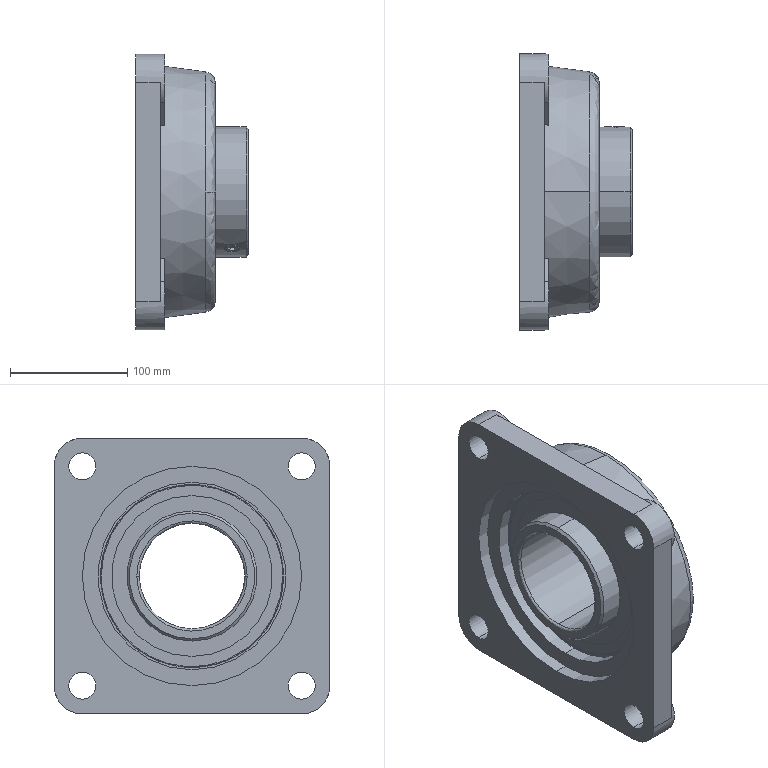Part | SolidWorks | 1 solid | 139 faces | box 96.3 x 235 x 235 mm | volume 1862383 mm3 | plane 49 | cylinder 48 | spline 22 | cone 20 | commonest cylinder face diameters 1.85 x8 23 x8 111 x8 48 x6 12 x4 137.163 x4